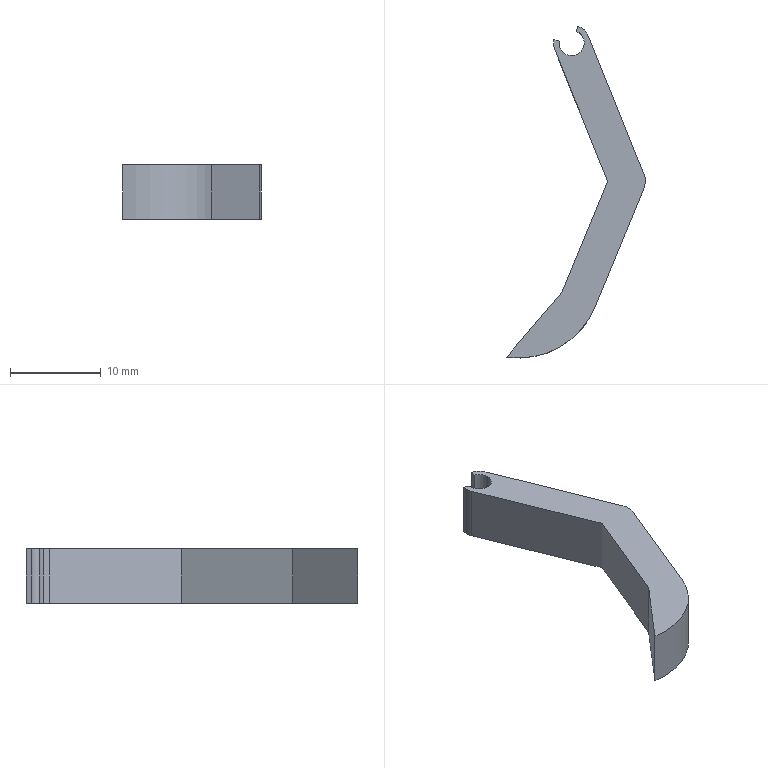Part | SolidWorks | features Extrusion 1 | 1 solid | 17 faces | box 15.303 x 36.626 x 6 mm | volume 919.383 mm3 | plane 9 | cylinder 8 | commonest cylinder face diameters 4 x4 2.773 x3 18.228 x1
STEP:
#1=CARTESIAN_POINT('',(13.438,-15.845,6.));
#2=VERTEX_POINT('',#1);
#3=CARTESIAN_POINT('',(13.583,-16.592,6.));
#4=VERTEX_POINT('',#3);
#5=CARTESIAN_POINT('',(15.438,-15.845,6.));
#6=DIRECTION('',(0.,0.,1.));
#7=DIRECTION('',(1.,0.,0.));
#8=AXIS2_PLACEMENT_3D('',#5,#6,#7);
#9=CIRCLE('',#8,2.);
#10=EDGE_CURVE('',#2,#4,#9,.T.);
#11=ORIENTED_EDGE('',*,*,#10,.F.);
#12=CARTESIAN_POINT('',(13.438,-15.845,0.));
#13=VERTEX_POINT('',#12);
#14=CARTESIAN_POINT('',(13.438,-15.845,6.));
#15=DIRECTION('',(0.,0.,-1.));
#16=VECTOR('',#15,1000.);
#17=LINE('',#14,#16);
#18=EDGE_CURVE('',#2,#13,#17,.T.);
#19=ORIENTED_EDGE('',*,*,#18,.T.);
#20=CARTESIAN_POINT('',(13.583,-16.592,0.));
#21=VERTEX_POINT('',#20);
#22=CARTESIAN_POINT('',(15.438,-15.845,0.));
#23=DIRECTION('',(0.,0.,1.));
#24=DIRECTION('',(1.,0.,0.));
#25=AXIS2_PLACEMENT_3D('',#22,#23,#24);
#26=CIRCLE('',#25,2.);
#27=EDGE_CURVE('',#13,#21,#26,.T.);
#28=ORIENTED_EDGE('',*,*,#27,.T.);
#29=CARTESIAN_POINT('',(13.583,-16.592,6.));
#30=DIRECTION('',(0.,0.,-1.));
#31=VECTOR('',#30,1000.);
#32=LINE('',#29,#31);
#33=EDGE_CURVE('',#4,#21,#32,.T.);
#34=ORIENTED_EDGE('',*,*,#33,.F.);
#35=EDGE_LOOP('',(#11,#19,#28,#34));
#36=FACE_OUTER_BOUND('',#35,.T.);
#37=CARTESIAN_POINT('',(15.438,-15.845,6.));
#38=DIRECTION('',(0.,0.,-1.));
#39=DIRECTION('',(-1.,0.,0.));
#40=AXIS2_PLACEMENT_3D('',#37,#38,#39);
#41=CYLINDRICAL_SURFACE('',#40,2.);
#42=ADVANCED_FACE('',(#36),#41,.T.);
#43=CARTESIAN_POINT('',(14.051,-15.845,6.));
#44=VERTEX_POINT('',#43);
#45=CARTESIAN_POINT('',(16.825,-15.845,6.));
#46=VERTEX_POINT('',#45);
#47=CARTESIAN_POINT('',(15.438,-15.845,6.));
#48=DIRECTION('',(0.,0.,1.));
#49=DIRECTION('',(1.,0.,0.));
#50=AXIS2_PLACEMENT_3D('',#47,#48,#49);
#51=CIRCLE('',#50,1.387);
#52=EDGE_CURVE('',#44,#46,#51,.T.);
#53=ORIENTED_EDGE('',*,*,#52,.T.);
#54=CARTESIAN_POINT('',(16.825,-15.845,0.));
#55=VERTEX_POINT('',#54);
#56=CARTESIAN_POINT('',(16.825,-15.845,6.));
#57=DIRECTION('',(0.,0.,-1.));
#58=VECTOR('',#57,1000.);
#59=LINE('',#56,#58);
#60=EDGE_CURVE('',#46,#55,#59,.T.);
#61=ORIENTED_EDGE('',*,*,#60,.T.);
#62=CARTESIAN_POINT('',(14.051,-15.845,0.));
#63=VERTEX_POINT('',#62);
#64=CARTESIAN_POINT('',(15.438,-15.845,0.));
#65=DIRECTION('',(0.,0.,1.));
#66=DIRECTION('',(1.,0.,0.));
#67=AXIS2_PLACEMENT_3D('',#64,#65,#66);
#68=CIRCLE('',#67,1.387);
#69=EDGE_CURVE('',#63,#55,#68,.T.);
#70=ORIENTED_EDGE('',*,*,#69,.F.);
#71=CARTESIAN_POINT('',(14.051,-15.845,6.));
#72=DIRECTION('',(0.,0.,-1.));
#73=VECTOR('',#72,1000.);
#74=LINE('',#71,#73);
#75=EDGE_CURVE('',#44,#63,#74,.T.);
#76=ORIENTED_EDGE('',*,*,#75,.F.);
#77=EDGE_LOOP('',(#53,#61,#70,#76));
#78=FACE_OUTER_BOUND('',#77,.T.);
#79=CARTESIAN_POINT('',(15.438,-15.845,6.));
#80=DIRECTION('',(0.,0.,-1.));
#81=DIRECTION('',(-1.,0.,0.));
#82=AXIS2_PLACEMENT_3D('',#79,#80,#81);
#83=CYLINDRICAL_SURFACE('',#82,1.387);
#84=ADVANCED_FACE('',(#78),#83,.F.);
#85=CARTESIAN_POINT('',(14.064,-15.659,6.));
#86=VERTEX_POINT('',#85);
#87=CARTESIAN_POINT('',(15.438,-15.845,6.));
#88=DIRECTION('',(0.,0.,1.));
#89=DIRECTION('',(1.,0.,0.));
#90=AXIS2_PLACEMENT_3D('',#87,#88,#89);
#91=CIRCLE('',#90,1.387);
#92=EDGE_CURVE('',#86,#44,#91,.T.);
#93=ORIENTED_EDGE('',*,*,#92,.T.);
#94=ORIENTED_EDGE('',*,*,#75,.T.);
#95=CARTESIAN_POINT('',(14.064,-15.659,0.));
#96=VERTEX_POINT('',#95);
#97=CARTESIAN_POINT('',(15.438,-15.845,0.));
#98=DIRECTION('',(0.,0.,1.));
#99=DIRECTION('',(1.,0.,0.));
#100=AXIS2_PLACEMENT_3D('',#97,#98,#99);
#101=CIRCLE('',#100,1.387);
#102=EDGE_CURVE('',#96,#63,#101,.T.);
#103=ORIENTED_EDGE('',*,*,#102,.F.);
#104=CARTESIAN_POINT('',(14.064,-15.659,6.));
#105=DIRECTION('',(0.,0.,-1.));
#106=VECTOR('',#105,1000.);
#107=LINE('',#104,#106);
#108=EDGE_CURVE('',#86,#96,#107,.T.);
#109=ORIENTED_EDGE('',*,*,#108,.F.);
#110=EDGE_LOOP('',(#93,#94,#103,#109));
#111=FACE_OUTER_BOUND('',#110,.T.);
#112=CARTESIAN_POINT('',(15.438,-15.845,6.));
#113=DIRECTION('',(0.,0.,-1.));
#114=DIRECTION('',(-1.,0.,0.));
#115=AXIS2_PLACEMENT_3D('',#112,#113,#114);
#116=CYLINDRICAL_SURFACE('',#115,1.387);
#117=ADVANCED_FACE('',(#111),#116,.F.);
#118=CARTESIAN_POINT('',(23.419,-31.84,0.));
#119=VERTEX_POINT('',#118);
#120=CARTESIAN_POINT('',(18.045,-44.93,0.));
#121=VERTEX_POINT('',#120);
#122=CARTESIAN_POINT('',(31.228,-12.822,0.));
#123=DIRECTION('',(-0.3798,-0.9251,0.));
#124=VECTOR('',#123,1000.);
#125=LINE('',#122,#124);
#126=EDGE_CURVE('',#119,#121,#125,.T.);
#127=ORIENTED_EDGE('',*,*,#126,.F.);
#128=CARTESIAN_POINT('',(23.419,-31.84,6.));
#129=VERTEX_POINT('',#128);
#130=CARTESIAN_POINT('',(23.419,-31.84,6.));
#131=DIRECTION('',(0.,0.,-1.));
#132=VECTOR('',#131,1000.);
#133=LINE('',#130,#132);
#134=EDGE_CURVE('',#129,#119,#133,.T.);
#135=ORIENTED_EDGE('',*,*,#134,.F.);
#136=CARTESIAN_POINT('',(18.045,-44.93,6.));
#137=VERTEX_POINT('',#136);
#138=CARTESIAN_POINT('',(31.228,-12.822,6.));
#139=DIRECTION('',(-0.3798,-0.9251,0.));
#140=VECTOR('',#139,1000.);
#141=LINE('',#138,#140);
#142=EDGE_CURVE('',#129,#137,#141,.T.);
#143=ORIENTED_EDGE('',*,*,#142,.T.);
#144=CARTESIAN_POINT('',(18.045,-44.93,6.));
#145=DIRECTION('',(0.,0.,-1.));
#146=VECTOR('',#145,1000.);
#147=LINE('',#144,#146);
#148=EDGE_CURVE('',#137,#121,#147,.T.);
#149=ORIENTED_EDGE('',*,*,#148,.T.);
#150=EDGE_LOOP('',(#127,#135,#143,#149));
#151=FACE_OUTER_BOUND('',#150,.T.);
#152=CARTESIAN_POINT('',(31.228,-12.822,6.));
#153=DIRECTION('',(0.9251,-0.3798,0.));
#154=DIRECTION('',(0.3798,0.9251,0.));
#155=AXIS2_PLACEMENT_3D('',#152,#153,#154);
#156=PLANE('',#155);
#157=ADVANCED_FACE('',(#151),#156,.T.);
#158=CARTESIAN_POINT('',(23.425,-30.334,0.));
#159=VERTEX_POINT('',#158);
#160=CARTESIAN_POINT('',(21.569,-31.081,0.));
#161=DIRECTION('',(0.,0.,1.));
#162=DIRECTION('',(1.,0.,0.));
#163=AXIS2_PLACEMENT_3D('',#160,#161,#162);
#164=CIRCLE('',#163,2.);
#165=EDGE_CURVE('',#119,#159,#164,.T.);
#166=ORIENTED_EDGE('',*,*,#165,.T.);
#167=CARTESIAN_POINT('',(23.425,-30.334,6.));
#168=VERTEX_POINT('',#167);
#169=CARTESIAN_POINT('',(23.425,-30.334,6.));
#170=DIRECTION('',(0.,0.,-1.));
#171=VECTOR('',#170,1000.);
#172=LINE('',#169,#171);
#173=EDGE_CURVE('',#168,#159,#172,.T.);
#174=ORIENTED_EDGE('',*,*,#173,.F.);
#175=CARTESIAN_POINT('',(21.569,-31.081,6.));
#176=DIRECTION('',(0.,0.,1.));
#177=DIRECTION('',(1.,0.,0.));
#178=AXIS2_PLACEMENT_3D('',#175,#176,#177);
#179=CIRCLE('',#178,2.);
#180=EDGE_CURVE('',#129,#168,#179,.T.);
#181=ORIENTED_EDGE('',*,*,#180,.F.);
#182=ORIENTED_EDGE('',*,*,#134,.T.);
#183=EDGE_LOOP('',(#166,#174,#181,#182));
#184=FACE_OUTER_BOUND('',#183,.T.);
#185=CARTESIAN_POINT('',(21.569,-31.081,6.));
#186=DIRECTION('',(0.,0.,-1.));
#187=DIRECTION('',(-1.,0.,0.));
#188=AXIS2_PLACEMENT_3D('',#185,#186,#187);
#189=CYLINDRICAL_SURFACE('',#188,2.);
#190=ADVANCED_FACE('',(#184),#189,.T.);
#191=CARTESIAN_POINT('',(17.294,-15.099,0.));
#192=VERTEX_POINT('',#191);
#193=CARTESIAN_POINT('',(9.654,3.885,0.));
#194=DIRECTION('',(0.3733,-0.9277,0.));
#195=VECTOR('',#194,1000.);
#196=LINE('',#193,#195);
#197=EDGE_CURVE('',#192,#159,#196,.T.);
#198=ORIENTED_EDGE('',*,*,#197,.F.);
#199=CARTESIAN_POINT('',(17.294,-15.099,6.));
#200=VERTEX_POINT('',#199);
#201=CARTESIAN_POINT('',(17.294,-15.099,6.));
#202=DIRECTION('',(0.,0.,-1.));
#203=VECTOR('',#202,1000.);
#204=LINE('',#201,#203);
#205=EDGE_CURVE('',#200,#192,#204,.T.);
#206=ORIENTED_EDGE('',*,*,#205,.F.);
#207=CARTESIAN_POINT('',(9.654,3.885,6.));
#208=DIRECTION('',(0.3733,-0.9277,0.));
#209=VECTOR('',#208,1000.);
#210=LINE('',#207,#209);
#211=EDGE_CURVE('',#200,#168,#210,.T.);
#212=ORIENTED_EDGE('',*,*,#211,.T.);
#213=ORIENTED_EDGE('',*,*,#173,.T.);
#214=EDGE_LOOP('',(#198,#206,#212,#213));
#215=FACE_OUTER_BOUND('',#214,.T.);
#216=CARTESIAN_POINT('',(9.654,3.885,6.));
#217=DIRECTION('',(0.9277,0.3733,0.));
#218=DIRECTION('',(-0.3733,0.9277,0.));
#219=AXIS2_PLACEMENT_3D('',#216,#217,#218);
#220=PLANE('',#219);
#221=ADVANCED_FACE('',(#215),#220,.T.);
#222=CARTESIAN_POINT('',(16.094,-13.956,0.));
#223=VERTEX_POINT('',#222);
#224=CARTESIAN_POINT('',(15.438,-15.845,0.));
#225=DIRECTION('',(0.,0.,1.));
#226=DIRECTION('',(1.,0.,0.));
#227=AXIS2_PLACEMENT_3D('',#224,#225,#226);
#228=CIRCLE('',#227,2.);
#229=EDGE_CURVE('',#192,#223,#228,.T.);
#230=ORIENTED_EDGE('',*,*,#229,.T.);
#231=CARTESIAN_POINT('',(16.094,-13.956,6.));
#232=VERTEX_POINT('',#231);
#233=CARTESIAN_POINT('',(16.094,-13.956,6.));
#234=DIRECTION('',(0.,0.,-1.));
#235=VECTOR('',#234,1000.);
#236=LINE('',#233,#235);
#237=EDGE_CURVE('',#232,#223,#236,.T.);
#238=ORIENTED_EDGE('',*,*,#237,.F.);
#239=CARTESIAN_POINT('',(15.438,-15.845,6.));
#240=DIRECTION('',(0.,0.,1.));
#241=DIRECTION('',(1.,0.,0.));
#242=AXIS2_PLACEMENT_3D('',#239,#240,#241);
#243=CIRCLE('',#242,2.);
#244=EDGE_CURVE('',#200,#232,#243,.T.);
#245=ORIENTED_EDGE('',*,*,#244,.F.);
#246=ORIENTED_EDGE('',*,*,#205,.T.);
#247=EDGE_LOOP('',(#230,#238,#245,#246));
#248=FACE_OUTER_BOUND('',#247,.T.);
#249=CARTESIAN_POINT('',(15.438,-15.845,6.));
#250=DIRECTION('',(0.,0.,-1.));
#251=DIRECTION('',(-1.,0.,0.));
#252=AXIS2_PLACEMENT_3D('',#249,#250,#251);
#253=CYLINDRICAL_SURFACE('',#252,2.);
#254=ADVANCED_FACE('',(#248),#253,.T.);
#255=CARTESIAN_POINT('',(15.963,-14.562,0.));
#256=VERTEX_POINT('',#255);
#257=CARTESIAN_POINT('',(18.263,-3.962,0.));
#258=DIRECTION('',(0.212,0.9773,0.));
#259=VECTOR('',#258,1000.);
#260=LINE('',#257,#259);
#261=EDGE_CURVE('',#256,#223,#260,.T.);
#262=ORIENTED_EDGE('',*,*,#261,.F.);
#263=CARTESIAN_POINT('',(15.963,-14.562,6.));
#264=VERTEX_POINT('',#263);
#265=CARTESIAN_POINT('',(15.963,-14.562,6.));
#266=DIRECTION('',(0.,0.,-1.));
#267=VECTOR('',#266,1000.);
#268=LINE('',#265,#267);
#269=EDGE_CURVE('',#264,#256,#268,.T.);
#270=ORIENTED_EDGE('',*,*,#269,.F.);
#271=CARTESIAN_POINT('',(18.263,-3.962,6.));
#272=DIRECTION('',(0.212,0.9773,0.));
#273=VECTOR('',#272,1000.);
#274=LINE('',#271,#273);
#275=EDGE_CURVE('',#264,#232,#274,.T.);
#276=ORIENTED_EDGE('',*,*,#275,.T.);
#277=ORIENTED_EDGE('',*,*,#237,.T.);
#278=EDGE_LOOP('',(#262,#270,#276,#277));
#279=FACE_OUTER_BOUND('',#278,.T.);
#280=CARTESIAN_POINT('',(18.263,-3.962,6.));
#281=DIRECTION('',(-0.9773,0.212,0.));
#282=DIRECTION('',(-0.212,-0.9773,0.));
#283=AXIS2_PLACEMENT_3D('',#280,#281,#282);
#284=PLANE('',#283);
#285=ADVANCED_FACE('',(#279),#284,.T.);
#286=ORIENTED_EDGE('',*,*,#60,.F.);
#287=CARTESIAN_POINT('',(15.438,-15.845,6.));
#288=DIRECTION('',(0.,0.,1.));
#289=DIRECTION('',(1.,0.,0.));
#290=AXIS2_PLACEMENT_3D('',#287,#288,#289);
#291=CIRCLE('',#290,1.387);
#292=EDGE_CURVE('',#46,#264,#291,.T.);
#293=ORIENTED_EDGE('',*,*,#292,.T.);
#294=ORIENTED_EDGE('',*,*,#269,.T.);
#295=CARTESIAN_POINT('',(15.438,-15.845,0.));
#296=DIRECTION('',(0.,0.,1.));
#297=DIRECTION('',(1.,0.,0.));
#298=AXIS2_PLACEMENT_3D('',#295,#296,#297);
#299=CIRCLE('',#298,1.387);
#300=EDGE_CURVE('',#55,#256,#299,.T.);
#301=ORIENTED_EDGE('',*,*,#300,.F.);
#302=EDGE_LOOP('',(#286,#293,#294,#301));
#303=FACE_OUTER_BOUND('',#302,.T.);
#304=CARTESIAN_POINT('',(15.438,-15.845,6.));
#305=DIRECTION('',(0.,0.,-1.));
#306=DIRECTION('',(-1.,0.,0.));
#307=AXIS2_PLACEMENT_3D('',#304,#305,#306);
#308=CYLINDRICAL_SURFACE('',#307,1.387);
#309=ADVANCED_FACE('',(#303),#308,.F.);
#310=CARTESIAN_POINT('',(13.484,-15.421,0.));
#311=VERTEX_POINT('',#310);
#312=CARTESIAN_POINT('',(-3.471,-8.488,0.));
#313=DIRECTION('',(-0.9256,0.3785,0.));
#314=VECTOR('',#313,1000.);
#315=LINE('',#312,#314);
#316=EDGE_CURVE('',#96,#311,#315,.T.);
#317=ORIENTED_EDGE('',*,*,#316,.T.);
#318=CARTESIAN_POINT('',(13.484,-15.421,6.));
#319=VERTEX_POINT('',#318);
#320=CARTESIAN_POINT('',(13.484,-15.421,6.));
#321=DIRECTION('',(0.,0.,-1.));
#322=VECTOR('',#321,1000.);
#323=LINE('',#320,#322);
#324=EDGE_CURVE('',#319,#311,#323,.T.);
#325=ORIENTED_EDGE('',*,*,#324,.F.);
#326=CARTESIAN_POINT('',(-3.471,-8.488,6.));
#327=DIRECTION('',(-0.9256,0.3785,0.));
#328=VECTOR('',#327,1000.);
#329=LINE('',#326,#328);
#330=EDGE_CURVE('',#86,#319,#329,.T.);
#331=ORIENTED_EDGE('',*,*,#330,.F.);
#332=ORIENTED_EDGE('',*,*,#108,.T.);
#333=EDGE_LOOP('',(#317,#325,#331,#332));
#334=FACE_OUTER_BOUND('',#333,.T.);
#335=CARTESIAN_POINT('',(-3.471,-8.488,6.));
#336=DIRECTION('',(-0.3785,-0.9256,0.));
#337=DIRECTION('',(0.9256,-0.3785,0.));
#338=AXIS2_PLACEMENT_3D('',#335,#336,#337);
#339=PLANE('',#338);
#340=ADVANCED_FACE('',(#334),#339,.F.);
#341=ORIENTED_EDGE('',*,*,#18,.F.);
#342=CARTESIAN_POINT('',(15.438,-15.845,6.));
#343=DIRECTION('',(0.,0.,1.));
#344=DIRECTION('',(1.,0.,0.));
#345=AXIS2_PLACEMENT_3D('',#342,#343,#344);
#346=CIRCLE('',#345,2.);
#347=EDGE_CURVE('',#319,#2,#346,.T.);
#348=ORIENTED_EDGE('',*,*,#347,.F.);
#349=ORIENTED_EDGE('',*,*,#324,.T.);
#350=CARTESIAN_POINT('',(15.438,-15.845,0.));
#351=DIRECTION('',(0.,0.,1.));
#352=DIRECTION('',(1.,0.,0.));
#353=AXIS2_PLACEMENT_3D('',#350,#351,#352);
#354=CIRCLE('',#353,2.);
#355=EDGE_CURVE('',#311,#13,#354,.T.);
#356=ORIENTED_EDGE('',*,*,#355,.T.);
#357=EDGE_LOOP('',(#341,#348,#349,#356));
#358=FACE_OUTER_BOUND('',#357,.T.);
#359=CARTESIAN_POINT('',(15.438,-15.845,6.));
#360=DIRECTION('',(0.,0.,-1.));
#361=DIRECTION('',(-1.,0.,0.));
#362=AXIS2_PLACEMENT_3D('',#359,#360,#361);
#363=CYLINDRICAL_SURFACE('',#362,2.);
#364=ADVANCED_FACE('',(#358),#363,.T.);
#365=CARTESIAN_POINT('',(19.41,-31.073,0.));
#366=VERTEX_POINT('',#365);
#367=CARTESIAN_POINT('',(5.943,2.392,0.));
#368=DIRECTION('',(0.3733,-0.9277,0.));
#369=VECTOR('',#368,1000.);
#370=LINE('',#367,#369);
#371=EDGE_CURVE('',#21,#366,#370,.T.);
#372=ORIENTED_EDGE('',*,*,#371,.T.);
#373=CARTESIAN_POINT('',(19.41,-31.073,6.));
#374=VERTEX_POINT('',#373);
#375=CARTESIAN_POINT('',(19.41,-31.073,6.));
#376=DIRECTION('',(0.,0.,-1.));
#377=VECTOR('',#376,1000.);
#378=LINE('',#375,#377);
#379=EDGE_CURVE('',#374,#366,#378,.T.);
#380=ORIENTED_EDGE('',*,*,#379,.F.);
#381=CARTESIAN_POINT('',(5.943,2.392,6.));
#382=DIRECTION('',(0.3733,-0.9277,0.));
#383=VECTOR('',#382,1000.);
#384=LINE('',#381,#383);
#385=EDGE_CURVE('',#4,#374,#384,.T.);
#386=ORIENTED_EDGE('',*,*,#385,.F.);
#387=ORIENTED_EDGE('',*,*,#33,.T.);
#388=EDGE_LOOP('',(#372,#380,#386,#387));
#389=FACE_OUTER_BOUND('',#388,.T.);
#390=CARTESIAN_POINT('',(5.943,2.392,6.));
#391=DIRECTION('',(0.9277,0.3733,0.));
#392=DIRECTION('',(-0.3733,0.9277,0.));
#393=AXIS2_PLACEMENT_3D('',#390,#391,#392);
#394=PLANE('',#393);
#395=ADVANCED_FACE('',(#389),#394,.F.);
#396=CARTESIAN_POINT('',(14.345,-43.41,0.));
#397=VERTEX_POINT('',#396);
#398=CARTESIAN_POINT('',(27.528,-11.302,0.));
#399=DIRECTION('',(-0.3798,-0.9251,0.));
#400=VECTOR('',#399,1000.);
#401=LINE('',#398,#400);
#402=EDGE_CURVE('',#366,#397,#401,.T.);
#403=ORIENTED_EDGE('',*,*,#402,.T.);
#404=CARTESIAN_POINT('',(14.345,-43.41,6.));
#405=VERTEX_POINT('',#404);
#406=CARTESIAN_POINT('',(14.345,-43.41,6.));
#407=DIRECTION('',(0.,0.,-1.));
#408=VECTOR('',#407,1000.);
#409=LINE('',#406,#408);
#410=EDGE_CURVE('',#405,#397,#409,.T.);
#411=ORIENTED_EDGE('',*,*,#410,.F.);
#412=CARTESIAN_POINT('',(27.528,-11.302,6.));
#413=DIRECTION('',(-0.3798,-0.9251,0.));
#414=VECTOR('',#413,1000.);
#415=LINE('',#412,#414);
#416=EDGE_CURVE('',#374,#405,#415,.T.);
#417=ORIENTED_EDGE('',*,*,#416,.F.);
#418=ORIENTED_EDGE('',*,*,#379,.T.);
#419=EDGE_LOOP('',(#403,#411,#417,#418));
#420=FACE_OUTER_BOUND('',#419,.T.);
#421=CARTESIAN_POINT('',(27.528,-11.302,6.));
#422=DIRECTION('',(0.9251,-0.3798,0.));
#423=DIRECTION('',(0.3798,0.9251,0.));
#424=AXIS2_PLACEMENT_3D('',#421,#422,#423);
#425=PLANE('',#424);
#426=ADVANCED_FACE('',(#420),#425,.F.);
#427=CARTESIAN_POINT('',(8.266,-50.482,0.));
#428=VERTEX_POINT('',#427);
#429=CARTESIAN_POINT('',(29.708,-25.539,0.));
#430=DIRECTION('',(-0.6519,-0.7583,0.));
#431=VECTOR('',#430,1000.);
#432=LINE('',#429,#431);
#433=EDGE_CURVE('',#397,#428,#432,.T.);
#434=ORIENTED_EDGE('',*,*,#433,.T.);
#435=CARTESIAN_POINT('',(8.266,-50.482,6.));
#436=VERTEX_POINT('',#435);
#437=CARTESIAN_POINT('',(8.266,-50.482,6.));
#438=DIRECTION('',(0.,0.,-1.));
#439=VECTOR('',#438,1000.);
#440=LINE('',#437,#439);
#441=EDGE_CURVE('',#436,#428,#440,.T.);
#442=ORIENTED_EDGE('',*,*,#441,.F.);
#443=CARTESIAN_POINT('',(29.708,-25.539,6.));
#444=DIRECTION('',(-0.6519,-0.7583,0.));
#445=VECTOR('',#444,1000.);
#446=LINE('',#443,#445);
#447=EDGE_CURVE('',#405,#436,#446,.T.);
#448=ORIENTED_EDGE('',*,*,#447,.F.);
#449=ORIENTED_EDGE('',*,*,#410,.T.);
#450=EDGE_LOOP('',(#434,#442,#448,#449));
#451=FACE_OUTER_BOUND('',#450,.T.);
#452=CARTESIAN_POINT('',(29.708,-25.539,6.));
#453=DIRECTION('',(0.7583,-0.6519,0.));
#454=DIRECTION('',(0.6519,0.7583,0.));
#455=AXIS2_PLACEMENT_3D('',#452,#453,#454);
#456=PLANE('',#455);
#457=ADVANCED_FACE('',(#451),#456,.F.);
#458=CARTESIAN_POINT('',(9.614,-41.468,0.));
#459=DIRECTION('',(0.,0.,1.));
#460=DIRECTION('',(1.,0.,0.));
#461=AXIS2_PLACEMENT_3D('',#458,#459,#460);
#462=CIRCLE('',#461,9.114);
#463=EDGE_CURVE('',#428,#121,#462,.T.);
#464=ORIENTED_EDGE('',*,*,#463,.T.);
#465=ORIENTED_EDGE('',*,*,#148,.F.);
#466=CARTESIAN_POINT('',(9.614,-41.468,6.));
#467=DIRECTION('',(0.,0.,1.));
#468=DIRECTION('',(1.,0.,0.));
#469=AXIS2_PLACEMENT_3D('',#466,#467,#468);
#470=CIRCLE('',#469,9.114);
#471=EDGE_CURVE('',#436,#137,#470,.T.);
#472=ORIENTED_EDGE('',*,*,#471,.F.);
#473=ORIENTED_EDGE('',*,*,#441,.T.);
#474=EDGE_LOOP('',(#464,#465,#472,#473));
#475=FACE_OUTER_BOUND('',#474,.T.);
#476=CARTESIAN_POINT('',(9.614,-41.468,6.));
#477=DIRECTION('',(0.,0.,-1.));
#478=DIRECTION('',(-1.,0.,0.));
#479=AXIS2_PLACEMENT_3D('',#476,#477,#478);
#480=CYLINDRICAL_SURFACE('',#479,9.114);
#481=ADVANCED_FACE('',(#475),#480,.T.);
#482=ORIENTED_EDGE('',*,*,#142,.F.);
#483=ORIENTED_EDGE('',*,*,#180,.T.);
#484=ORIENTED_EDGE('',*,*,#211,.F.);
#485=ORIENTED_EDGE('',*,*,#244,.T.);
#486=ORIENTED_EDGE('',*,*,#275,.F.);
#487=ORIENTED_EDGE('',*,*,#292,.F.);
#488=ORIENTED_EDGE('',*,*,#52,.F.);
#489=ORIENTED_EDGE('',*,*,#92,.F.);
#490=ORIENTED_EDGE('',*,*,#330,.T.);
#491=ORIENTED_EDGE('',*,*,#347,.T.);
#492=ORIENTED_EDGE('',*,*,#10,.T.);
#493=ORIENTED_EDGE('',*,*,#385,.T.);
#494=ORIENTED_EDGE('',*,*,#416,.T.);
#495=ORIENTED_EDGE('',*,*,#447,.T.);
#496=ORIENTED_EDGE('',*,*,#471,.T.);
#497=EDGE_LOOP('',(#482,#483,#484,#485,#486,#487,#488,#489,#490,#491,#492,#493,#494,#495,#496));
#498=FACE_OUTER_BOUND('',#497,.T.);
#499=CARTESIAN_POINT('',(0.,0.,6.));
#500=DIRECTION('',(0.,0.,1.));
#501=DIRECTION('',(1.,0.,0.));
#502=AXIS2_PLACEMENT_3D('',#499,#500,#501);
#503=PLANE('',#502);
#504=ADVANCED_FACE('',(#498),#503,.T.);
#505=ORIENTED_EDGE('',*,*,#126,.T.);
#506=ORIENTED_EDGE('',*,*,#463,.F.);
#507=ORIENTED_EDGE('',*,*,#433,.F.);
#508=ORIENTED_EDGE('',*,*,#402,.F.);
#509=ORIENTED_EDGE('',*,*,#371,.F.);
#510=ORIENTED_EDGE('',*,*,#27,.F.);
#511=ORIENTED_EDGE('',*,*,#355,.F.);
#512=ORIENTED_EDGE('',*,*,#316,.F.);
#513=ORIENTED_EDGE('',*,*,#102,.T.);
#514=ORIENTED_EDGE('',*,*,#69,.T.);
#515=ORIENTED_EDGE('',*,*,#300,.T.);
#516=ORIENTED_EDGE('',*,*,#261,.T.);
#517=ORIENTED_EDGE('',*,*,#229,.F.);
#518=ORIENTED_EDGE('',*,*,#197,.T.);
#519=ORIENTED_EDGE('',*,*,#165,.F.);
#520=EDGE_LOOP('',(#505,#506,#507,#508,#509,#510,#511,#512,#513,#514,#515,#516,#517,#518,#519));
#521=FACE_OUTER_BOUND('',#520,.T.);
#522=CARTESIAN_POINT('',(0.,0.,0.));
#523=DIRECTION('',(0.,0.,1.));
#524=DIRECTION('',(1.,0.,0.));
#525=AXIS2_PLACEMENT_3D('',#522,#523,#524);
#526=PLANE('',#525);
#527=ADVANCED_FACE('',(#521),#526,.F.);
#528=CLOSED_SHELL('',(#42,#84,#117,#157,#190,#221,#254,#285,#309,#340,#364,#395,#426,#457,#481,#504,#527));
#529=MANIFOLD_SOLID_BREP('',#528);
#530=CARTESIAN_POINT('',(0.,0.,0.));
#531=DIRECTION('',(0.,0.,1.));
#532=DIRECTION('',(1.,0.,0.));
#533=AXIS2_PLACEMENT_3D('',#530,#531,#532);
#534=(LENGTH_UNIT()NAMED_UNIT(*)SI_UNIT(.MILLI.,.METRE.));
#535=UNCERTAINTY_MEASURE_WITH_UNIT(LENGTH_MEASURE(0.00001),#534,'','');
#536=(NAMED_UNIT(*)PLANE_ANGLE_UNIT()SI_UNIT($,.RADIAN.));
#537=(NAMED_UNIT(*)SI_UNIT($,.STERADIAN.)SOLID_ANGLE_UNIT());
#538=(GEOMETRIC_REPRESENTATION_CONTEXT(3)GLOBAL_UNCERTAINTY_ASSIGNED_CONTEXT((#535))GLOBAL_UNIT_ASSIGNED_CONTEXT((#534,#536,#537))REPRESENTATION_CONTEXT('',''));
#539=ADVANCED_BREP_SHAPE_REPRESENTATION('',(#529,#533),#538);